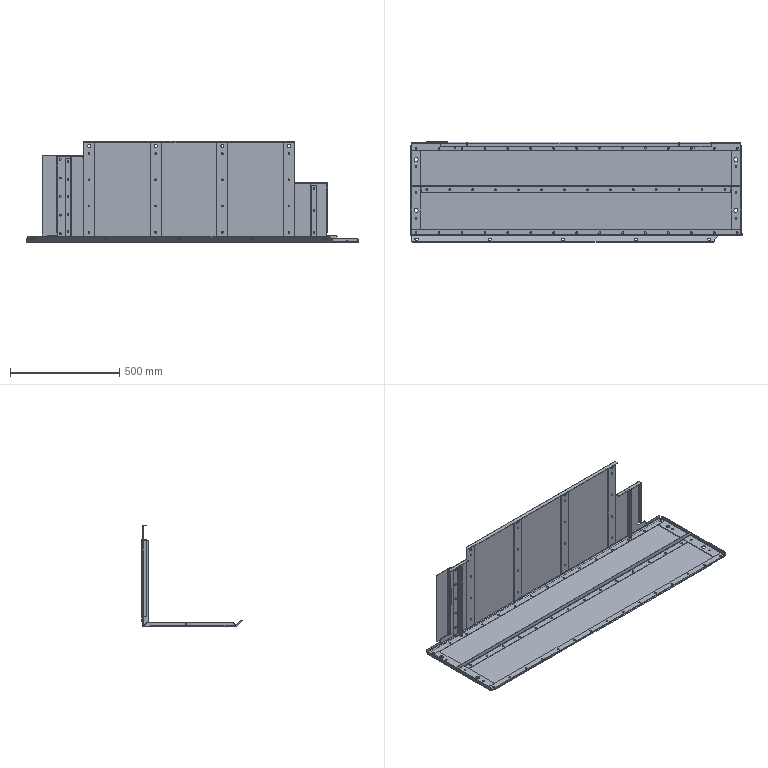Part | SolidWorks | features ReferencePattern 3, CompositeCurve 1, LocalLPattern 1 | 13 solids | 457 faces | box 1520 x 459.004 x 465.1 mm | volume 3224415 mm3 | cylinder 268 | plane 184 | spline 5 | commonest cylinder face diameters 8 x164 15 x26 10 x19 18 x16 5 x11 9 x11